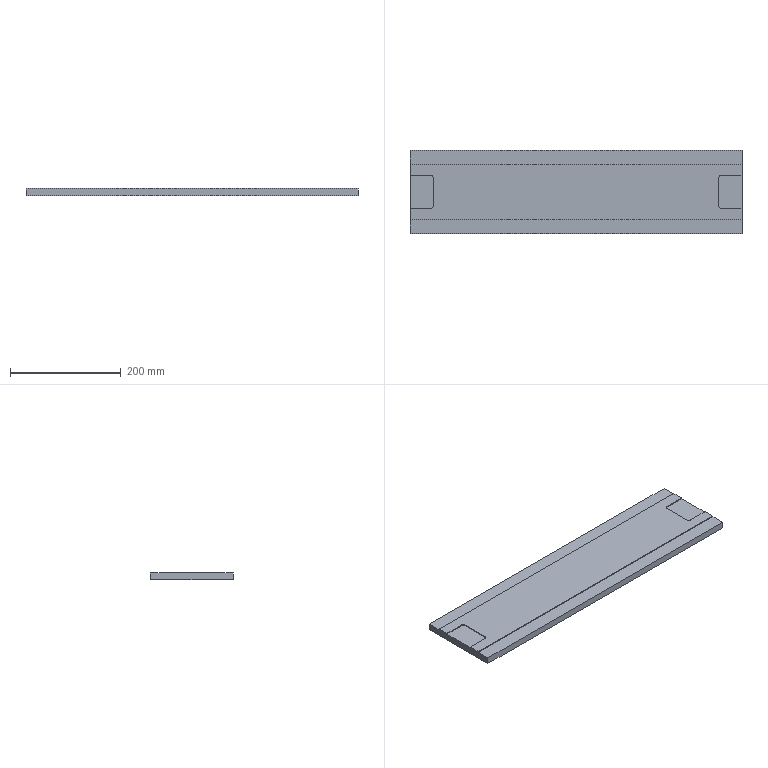Part | SolidWorks | features ICE 3, Extrusion 1, Fillet 1 | 1 solid | 22 faces | box 600 x 150 x 14 mm | volume 1207472 mm3 | plane 18 | cylinder 4 | commonest cylinder face diameters 10 x4
STEP:
#1=CARTESIAN_POINT('',(300.,75.,12.5));
#2=VERTEX_POINT('',#1);
#3=CARTESIAN_POINT('',(-300.,75.,12.5));
#4=VERTEX_POINT('',#3);
#5=CARTESIAN_POINT('',(-300.,75.,12.5));
#6=DIRECTION('',(-1.,0.,0.));
#7=VECTOR('',#6,1000.);
#8=LINE('',#5,#7);
#9=EDGE_CURVE('',#2,#4,#8,.T.);
#10=ORIENTED_EDGE('',*,*,#9,.F.);
#11=CARTESIAN_POINT('',(300.,75.,0.));
#12=VERTEX_POINT('',#11);
#13=CARTESIAN_POINT('',(300.,75.,14.));
#14=DIRECTION('',(0.,0.,-1.));
#15=VECTOR('',#14,1000.);
#16=LINE('',#13,#15);
#17=EDGE_CURVE('',#2,#12,#16,.T.);
#18=ORIENTED_EDGE('',*,*,#17,.T.);
#19=CARTESIAN_POINT('',(-300.,75.,0.));
#20=VERTEX_POINT('',#19);
#21=CARTESIAN_POINT('',(-300.,75.,0.));
#22=DIRECTION('',(-1.,0.,0.));
#23=VECTOR('',#22,1000.);
#24=LINE('',#21,#23);
#25=EDGE_CURVE('',#12,#20,#24,.T.);
#26=ORIENTED_EDGE('',*,*,#25,.T.);
#27=CARTESIAN_POINT('',(-300.,75.,14.));
#28=DIRECTION('',(0.,0.,-1.));
#29=VECTOR('',#28,1000.);
#30=LINE('',#27,#29);
#31=EDGE_CURVE('',#4,#20,#30,.T.);
#32=ORIENTED_EDGE('',*,*,#31,.F.);
#33=EDGE_LOOP('',(#10,#18,#26,#32));
#34=FACE_OUTER_BOUND('',#33,.T.);
#35=CARTESIAN_POINT('',(-300.,75.,14.));
#36=DIRECTION('',(0.,-1.,0.));
#37=DIRECTION('',(0.,0.,-1.));
#38=AXIS2_PLACEMENT_3D('',#35,#36,#37);
#39=PLANE('',#38);
#40=ADVANCED_FACE('',(#34),#39,.F.);
#41=CARTESIAN_POINT('',(300.,-30.,12.5));
#42=VERTEX_POINT('',#41);
#43=CARTESIAN_POINT('',(300.,30.,12.5));
#44=VERTEX_POINT('',#43);
#45=CARTESIAN_POINT('',(300.,-30.,12.5));
#46=DIRECTION('',(0.,1.,0.));
#47=VECTOR('',#46,1000.);
#48=LINE('',#45,#47);
#49=EDGE_CURVE('',#42,#44,#48,.T.);
#50=ORIENTED_EDGE('',*,*,#49,.F.);
#51=CARTESIAN_POINT('',(300.,-30.,14.));
#52=VERTEX_POINT('',#51);
#53=CARTESIAN_POINT('',(300.,-30.,12.5));
#54=DIRECTION('',(0.,0.,1.));
#55=VECTOR('',#54,1000.);
#56=LINE('',#53,#55);
#57=EDGE_CURVE('',#42,#52,#56,.T.);
#58=ORIENTED_EDGE('',*,*,#57,.T.);
#59=CARTESIAN_POINT('',(300.,-50.,14.));
#60=VERTEX_POINT('',#59);
#61=CARTESIAN_POINT('',(300.,-75.,14.));
#62=DIRECTION('',(0.,1.,0.));
#63=VECTOR('',#62,1000.);
#64=LINE('',#61,#63);
#65=EDGE_CURVE('',#60,#52,#64,.T.);
#66=ORIENTED_EDGE('',*,*,#65,.F.);
#67=CARTESIAN_POINT('',(300.,-50.,12.5));
#68=VERTEX_POINT('',#67);
#69=CARTESIAN_POINT('',(300.,-50.,12.5));
#70=DIRECTION('',(0.,0.,1.));
#71=VECTOR('',#70,1000.);
#72=LINE('',#69,#71);
#73=EDGE_CURVE('',#68,#60,#72,.T.);
#74=ORIENTED_EDGE('',*,*,#73,.F.);
#75=CARTESIAN_POINT('',(300.,-75.,12.5));
#76=VERTEX_POINT('',#75);
#77=CARTESIAN_POINT('',(300.,-75.,12.5));
#78=DIRECTION('',(0.,1.,0.));
#79=VECTOR('',#78,1000.);
#80=LINE('',#77,#79);
#81=EDGE_CURVE('',#76,#68,#80,.T.);
#82=ORIENTED_EDGE('',*,*,#81,.F.);
#83=CARTESIAN_POINT('',(300.,-75.,0.));
#84=VERTEX_POINT('',#83);
#85=CARTESIAN_POINT('',(300.,-75.,14.));
#86=DIRECTION('',(0.,0.,-1.));
#87=VECTOR('',#86,1000.);
#88=LINE('',#85,#87);
#89=EDGE_CURVE('',#76,#84,#88,.T.);
#90=ORIENTED_EDGE('',*,*,#89,.T.);
#91=CARTESIAN_POINT('',(300.,-75.,0.));
#92=DIRECTION('',(0.,1.,0.));
#93=VECTOR('',#92,1000.);
#94=LINE('',#91,#93);
#95=EDGE_CURVE('',#84,#12,#94,.T.);
#96=ORIENTED_EDGE('',*,*,#95,.T.);
#97=ORIENTED_EDGE('',*,*,#17,.F.);
#98=CARTESIAN_POINT('',(300.,50.,12.5));
#99=VERTEX_POINT('',#98);
#100=CARTESIAN_POINT('',(300.,75.,12.5));
#101=DIRECTION('',(0.,1.,0.));
#102=VECTOR('',#101,1000.);
#103=LINE('',#100,#102);
#104=EDGE_CURVE('',#99,#2,#103,.T.);
#105=ORIENTED_EDGE('',*,*,#104,.F.);
#106=CARTESIAN_POINT('',(300.,50.,14.));
#107=VERTEX_POINT('',#106);
#108=CARTESIAN_POINT('',(300.,50.,12.5));
#109=DIRECTION('',(0.,0.,1.));
#110=VECTOR('',#109,1000.);
#111=LINE('',#108,#110);
#112=EDGE_CURVE('',#99,#107,#111,.T.);
#113=ORIENTED_EDGE('',*,*,#112,.T.);
#114=CARTESIAN_POINT('',(300.,30.,14.));
#115=VERTEX_POINT('',#114);
#116=CARTESIAN_POINT('',(300.,-75.,14.));
#117=DIRECTION('',(0.,1.,0.));
#118=VECTOR('',#117,1000.);
#119=LINE('',#116,#118);
#120=EDGE_CURVE('',#115,#107,#119,.T.);
#121=ORIENTED_EDGE('',*,*,#120,.F.);
#122=CARTESIAN_POINT('',(300.,30.,12.5));
#123=DIRECTION('',(0.,0.,1.));
#124=VECTOR('',#123,1000.);
#125=LINE('',#122,#124);
#126=EDGE_CURVE('',#44,#115,#125,.T.);
#127=ORIENTED_EDGE('',*,*,#126,.F.);
#128=EDGE_LOOP('',(#50,#58,#66,#74,#82,#90,#96,#97,#105,#113,#121,#127));
#129=FACE_OUTER_BOUND('',#128,.T.);
#130=CARTESIAN_POINT('',(300.,-75.,14.));
#131=DIRECTION('',(-1.,0.,0.));
#132=DIRECTION('',(0.,0.,1.));
#133=AXIS2_PLACEMENT_3D('',#130,#131,#132);
#134=PLANE('',#133);
#135=ADVANCED_FACE('',(#129),#134,.F.);
#136=CARTESIAN_POINT('',(-300.,-30.,14.));
#137=VERTEX_POINT('',#136);
#138=CARTESIAN_POINT('',(-300.,-50.,14.));
#139=VERTEX_POINT('',#138);
#140=CARTESIAN_POINT('',(-300.,-75.,14.));
#141=DIRECTION('',(0.,-1.,0.));
#142=VECTOR('',#141,1000.);
#143=LINE('',#140,#142);
#144=EDGE_CURVE('',#137,#139,#143,.T.);
#145=ORIENTED_EDGE('',*,*,#144,.F.);
#146=CARTESIAN_POINT('',(-300.,-30.,12.5));
#147=VERTEX_POINT('',#146);
#148=CARTESIAN_POINT('',(-300.,-30.,12.5));
#149=DIRECTION('',(0.,0.,1.));
#150=VECTOR('',#149,1000.);
#151=LINE('',#148,#150);
#152=EDGE_CURVE('',#147,#137,#151,.T.);
#153=ORIENTED_EDGE('',*,*,#152,.F.);
#154=CARTESIAN_POINT('',(-300.,30.,12.5));
#155=VERTEX_POINT('',#154);
#156=CARTESIAN_POINT('',(-300.,-30.,12.5));
#157=DIRECTION('',(0.,-1.,0.));
#158=VECTOR('',#157,1000.);
#159=LINE('',#156,#158);
#160=EDGE_CURVE('',#155,#147,#159,.T.);
#161=ORIENTED_EDGE('',*,*,#160,.F.);
#162=CARTESIAN_POINT('',(-300.,30.,14.));
#163=VERTEX_POINT('',#162);
#164=CARTESIAN_POINT('',(-300.,30.,12.5));
#165=DIRECTION('',(0.,0.,1.));
#166=VECTOR('',#165,1000.);
#167=LINE('',#164,#166);
#168=EDGE_CURVE('',#155,#163,#167,.T.);
#169=ORIENTED_EDGE('',*,*,#168,.T.);
#170=CARTESIAN_POINT('',(-300.,50.,14.));
#171=VERTEX_POINT('',#170);
#172=CARTESIAN_POINT('',(-300.,-75.,14.));
#173=DIRECTION('',(0.,-1.,0.));
#174=VECTOR('',#173,1000.);
#175=LINE('',#172,#174);
#176=EDGE_CURVE('',#171,#163,#175,.T.);
#177=ORIENTED_EDGE('',*,*,#176,.F.);
#178=CARTESIAN_POINT('',(-300.,50.,12.5));
#179=VERTEX_POINT('',#178);
#180=CARTESIAN_POINT('',(-300.,50.,12.5));
#181=DIRECTION('',(0.,0.,1.));
#182=VECTOR('',#181,1000.);
#183=LINE('',#180,#182);
#184=EDGE_CURVE('',#179,#171,#183,.T.);
#185=ORIENTED_EDGE('',*,*,#184,.F.);
#186=CARTESIAN_POINT('',(-300.,75.,12.5));
#187=DIRECTION('',(0.,-1.,0.));
#188=VECTOR('',#187,1000.);
#189=LINE('',#186,#188);
#190=EDGE_CURVE('',#4,#179,#189,.T.);
#191=ORIENTED_EDGE('',*,*,#190,.F.);
#192=ORIENTED_EDGE('',*,*,#31,.T.);
#193=CARTESIAN_POINT('',(-300.,-75.,0.));
#194=VERTEX_POINT('',#193);
#195=CARTESIAN_POINT('',(-300.,-75.,0.));
#196=DIRECTION('',(0.,-1.,0.));
#197=VECTOR('',#196,1000.);
#198=LINE('',#195,#197);
#199=EDGE_CURVE('',#20,#194,#198,.T.);
#200=ORIENTED_EDGE('',*,*,#199,.T.);
#201=CARTESIAN_POINT('',(-300.,-75.,12.5));
#202=VERTEX_POINT('',#201);
#203=CARTESIAN_POINT('',(-300.,-75.,14.));
#204=DIRECTION('',(0.,0.,-1.));
#205=VECTOR('',#204,1000.);
#206=LINE('',#203,#205);
#207=EDGE_CURVE('',#202,#194,#206,.T.);
#208=ORIENTED_EDGE('',*,*,#207,.F.);
#209=CARTESIAN_POINT('',(-300.,-50.,12.5));
#210=VERTEX_POINT('',#209);
#211=CARTESIAN_POINT('',(-300.,-75.,12.5));
#212=DIRECTION('',(0.,-1.,0.));
#213=VECTOR('',#212,1000.);
#214=LINE('',#211,#213);
#215=EDGE_CURVE('',#210,#202,#214,.T.);
#216=ORIENTED_EDGE('',*,*,#215,.F.);
#217=CARTESIAN_POINT('',(-300.,-50.,12.5));
#218=DIRECTION('',(0.,0.,1.));
#219=VECTOR('',#218,1000.);
#220=LINE('',#217,#219);
#221=EDGE_CURVE('',#210,#139,#220,.T.);
#222=ORIENTED_EDGE('',*,*,#221,.T.);
#223=EDGE_LOOP('',(#145,#153,#161,#169,#177,#185,#191,#192,#200,#208,#216,#222));
#224=FACE_OUTER_BOUND('',#223,.T.);
#225=CARTESIAN_POINT('',(-300.,-75.,14.));
#226=DIRECTION('',(1.,0.,0.));
#227=DIRECTION('',(0.,0.,-1.));
#228=AXIS2_PLACEMENT_3D('',#225,#226,#227);
#229=PLANE('',#228);
#230=ADVANCED_FACE('',(#224),#229,.F.);
#231=ORIENTED_EDGE('',*,*,#89,.F.);
#232=CARTESIAN_POINT('',(-300.,-75.,12.5));
#233=DIRECTION('',(1.,0.,0.));
#234=VECTOR('',#233,1000.);
#235=LINE('',#232,#234);
#236=EDGE_CURVE('',#202,#76,#235,.T.);
#237=ORIENTED_EDGE('',*,*,#236,.F.);
#238=ORIENTED_EDGE('',*,*,#207,.T.);
#239=CARTESIAN_POINT('',(-300.,-75.,0.));
#240=DIRECTION('',(1.,0.,0.));
#241=VECTOR('',#240,1000.);
#242=LINE('',#239,#241);
#243=EDGE_CURVE('',#194,#84,#242,.T.);
#244=ORIENTED_EDGE('',*,*,#243,.T.);
#245=EDGE_LOOP('',(#231,#237,#238,#244));
#246=FACE_OUTER_BOUND('',#245,.T.);
#247=CARTESIAN_POINT('',(-300.,-75.,14.));
#248=DIRECTION('',(0.,1.,0.));
#249=DIRECTION('',(0.,0.,1.));
#250=AXIS2_PLACEMENT_3D('',#247,#248,#249);
#251=PLANE('',#250);
#252=ADVANCED_FACE('',(#246),#251,.F.);
#253=CARTESIAN_POINT('',(-258.,-25.,14.));
#254=VERTEX_POINT('',#253);
#255=CARTESIAN_POINT('',(-258.,25.,14.));
#256=VERTEX_POINT('',#255);
#257=CARTESIAN_POINT('',(-258.,-30.,14.));
#258=DIRECTION('',(0.,1.,0.));
#259=VECTOR('',#258,1000.);
#260=LINE('',#257,#259);
#261=EDGE_CURVE('',#254,#256,#260,.T.);
#262=ORIENTED_EDGE('',*,*,#261,.F.);
#263=CARTESIAN_POINT('',(-263.,-30.,14.));
#264=VERTEX_POINT('',#263);
#265=CARTESIAN_POINT('',(-263.,-25.,14.));
#266=DIRECTION('',(0.,0.,-1.));
#267=DIRECTION('',(-1.,0.,0.));
#268=AXIS2_PLACEMENT_3D('',#265,#266,#267);
#269=CIRCLE('',#268,5.);
#270=EDGE_CURVE('',#254,#264,#269,.T.);
#271=ORIENTED_EDGE('',*,*,#270,.T.);
#272=CARTESIAN_POINT('',(-300.,-30.,14.));
#273=DIRECTION('',(1.,0.,0.));
#274=VECTOR('',#273,1000.);
#275=LINE('',#272,#274);
#276=EDGE_CURVE('',#137,#264,#275,.T.);
#277=ORIENTED_EDGE('',*,*,#276,.F.);
#278=ORIENTED_EDGE('',*,*,#144,.T.);
#279=CARTESIAN_POINT('',(-300.,-50.,14.));
#280=DIRECTION('',(-1.,0.,0.));
#281=VECTOR('',#280,1000.);
#282=LINE('',#279,#281);
#283=EDGE_CURVE('',#60,#139,#282,.T.);
#284=ORIENTED_EDGE('',*,*,#283,.F.);
#285=ORIENTED_EDGE('',*,*,#65,.T.);
#286=CARTESIAN_POINT('',(263.,-30.,14.));
#287=VERTEX_POINT('',#286);
#288=CARTESIAN_POINT('',(258.,-30.,14.));
#289=DIRECTION('',(1.,0.,0.));
#290=VECTOR('',#289,1000.);
#291=LINE('',#288,#290);
#292=EDGE_CURVE('',#287,#52,#291,.T.);
#293=ORIENTED_EDGE('',*,*,#292,.F.);
#294=CARTESIAN_POINT('',(258.,-25.,14.));
#295=VERTEX_POINT('',#294);
#296=CARTESIAN_POINT('',(263.,-25.,14.));
#297=DIRECTION('',(0.,0.,-1.));
#298=DIRECTION('',(-1.,0.,0.));
#299=AXIS2_PLACEMENT_3D('',#296,#297,#298);
#300=CIRCLE('',#299,5.);
#301=EDGE_CURVE('',#287,#295,#300,.T.);
#302=ORIENTED_EDGE('',*,*,#301,.T.);
#303=CARTESIAN_POINT('',(258.,25.,14.));
#304=VERTEX_POINT('',#303);
#305=CARTESIAN_POINT('',(258.,-30.,14.));
#306=DIRECTION('',(0.,-1.,0.));
#307=VECTOR('',#306,1000.);
#308=LINE('',#305,#307);
#309=EDGE_CURVE('',#304,#295,#308,.T.);
#310=ORIENTED_EDGE('',*,*,#309,.F.);
#311=CARTESIAN_POINT('',(263.,30.,14.));
#312=VERTEX_POINT('',#311);
#313=CARTESIAN_POINT('',(263.,25.,14.));
#314=DIRECTION('',(0.,0.,-1.));
#315=DIRECTION('',(-1.,0.,0.));
#316=AXIS2_PLACEMENT_3D('',#313,#314,#315);
#317=CIRCLE('',#316,5.);
#318=EDGE_CURVE('',#304,#312,#317,.T.);
#319=ORIENTED_EDGE('',*,*,#318,.T.);
#320=CARTESIAN_POINT('',(258.,30.,14.));
#321=DIRECTION('',(-1.,0.,0.));
#322=VECTOR('',#321,1000.);
#323=LINE('',#320,#322);
#324=EDGE_CURVE('',#115,#312,#323,.T.);
#325=ORIENTED_EDGE('',*,*,#324,.F.);
#326=ORIENTED_EDGE('',*,*,#120,.T.);
#327=CARTESIAN_POINT('',(-300.,50.,14.));
#328=DIRECTION('',(1.,0.,0.));
#329=VECTOR('',#328,1000.);
#330=LINE('',#327,#329);
#331=EDGE_CURVE('',#171,#107,#330,.T.);
#332=ORIENTED_EDGE('',*,*,#331,.F.);
#333=ORIENTED_EDGE('',*,*,#176,.T.);
#334=CARTESIAN_POINT('',(-263.,30.,14.));
#335=VERTEX_POINT('',#334);
#336=CARTESIAN_POINT('',(-300.,30.,14.));
#337=DIRECTION('',(-1.,0.,0.));
#338=VECTOR('',#337,1000.);
#339=LINE('',#336,#338);
#340=EDGE_CURVE('',#335,#163,#339,.T.);
#341=ORIENTED_EDGE('',*,*,#340,.F.);
#342=CARTESIAN_POINT('',(-263.,25.,14.));
#343=DIRECTION('',(0.,0.,-1.));
#344=DIRECTION('',(-1.,0.,0.));
#345=AXIS2_PLACEMENT_3D('',#342,#343,#344);
#346=CIRCLE('',#345,5.);
#347=EDGE_CURVE('',#335,#256,#346,.T.);
#348=ORIENTED_EDGE('',*,*,#347,.T.);
#349=EDGE_LOOP('',(#262,#271,#277,#278,#284,#285,#293,#302,#310,#319,#325,#326,#332,#333,#341,#348));
#350=FACE_OUTER_BOUND('',#349,.T.);
#351=CARTESIAN_POINT('',(0.,0.,14.));
#352=DIRECTION('',(0.,0.,-1.));
#353=DIRECTION('',(-1.,0.,0.));
#354=AXIS2_PLACEMENT_3D('',#351,#352,#353);
#355=PLANE('',#354);
#356=ADVANCED_FACE('',(#350),#355,.F.);
#357=ORIENTED_EDGE('',*,*,#95,.F.);
#358=ORIENTED_EDGE('',*,*,#243,.F.);
#359=ORIENTED_EDGE('',*,*,#199,.F.);
#360=ORIENTED_EDGE('',*,*,#25,.F.);
#361=EDGE_LOOP('',(#357,#358,#359,#360));
#362=FACE_OUTER_BOUND('',#361,.T.);
#363=CARTESIAN_POINT('',(0.,0.,0.));
#364=DIRECTION('',(0.,0.,-1.));
#365=DIRECTION('',(-1.,0.,0.));
#366=AXIS2_PLACEMENT_3D('',#363,#364,#365);
#367=PLANE('',#366);
#368=ADVANCED_FACE('',(#362),#367,.T.);
#369=ORIENTED_EDGE('',*,*,#283,.T.);
#370=ORIENTED_EDGE('',*,*,#221,.F.);
#371=CARTESIAN_POINT('',(-300.,-50.,12.5));
#372=DIRECTION('',(-1.,0.,0.));
#373=VECTOR('',#372,1000.);
#374=LINE('',#371,#373);
#375=EDGE_CURVE('',#68,#210,#374,.T.);
#376=ORIENTED_EDGE('',*,*,#375,.F.);
#377=ORIENTED_EDGE('',*,*,#73,.T.);
#378=EDGE_LOOP('',(#369,#370,#376,#377));
#379=FACE_OUTER_BOUND('',#378,.T.);
#380=CARTESIAN_POINT('',(-300.,-50.,12.5));
#381=DIRECTION('',(0.,1.,0.));
#382=DIRECTION('',(-1.,0.,0.));
#383=AXIS2_PLACEMENT_3D('',#380,#381,#382);
#384=PLANE('',#383);
#385=ADVANCED_FACE('',(#379),#384,.F.);
#386=ORIENTED_EDGE('',*,*,#215,.T.);
#387=ORIENTED_EDGE('',*,*,#236,.T.);
#388=ORIENTED_EDGE('',*,*,#81,.T.);
#389=ORIENTED_EDGE('',*,*,#375,.T.);
#390=EDGE_LOOP('',(#386,#387,#388,#389));
#391=FACE_OUTER_BOUND('',#390,.T.);
#392=CARTESIAN_POINT('',(0.,0.,12.5));
#393=DIRECTION('',(0.,0.,-1.));
#394=DIRECTION('',(-1.,0.,0.));
#395=AXIS2_PLACEMENT_3D('',#392,#393,#394);
#396=PLANE('',#395);
#397=ADVANCED_FACE('',(#391),#396,.F.);
#398=ORIENTED_EDGE('',*,*,#331,.T.);
#399=ORIENTED_EDGE('',*,*,#112,.F.);
#400=CARTESIAN_POINT('',(-300.,50.,12.5));
#401=DIRECTION('',(1.,0.,0.));
#402=VECTOR('',#401,1000.);
#403=LINE('',#400,#402);
#404=EDGE_CURVE('',#179,#99,#403,.T.);
#405=ORIENTED_EDGE('',*,*,#404,.F.);
#406=ORIENTED_EDGE('',*,*,#184,.T.);
#407=EDGE_LOOP('',(#398,#399,#405,#406));
#408=FACE_OUTER_BOUND('',#407,.T.);
#409=CARTESIAN_POINT('',(-300.,50.,12.5));
#410=DIRECTION('',(0.,-1.,0.));
#411=DIRECTION('',(0.,0.,-1.));
#412=AXIS2_PLACEMENT_3D('',#409,#410,#411);
#413=PLANE('',#412);
#414=ADVANCED_FACE('',(#408),#413,.F.);
#415=ORIENTED_EDGE('',*,*,#190,.T.);
#416=ORIENTED_EDGE('',*,*,#404,.T.);
#417=ORIENTED_EDGE('',*,*,#104,.T.);
#418=ORIENTED_EDGE('',*,*,#9,.T.);
#419=EDGE_LOOP('',(#415,#416,#417,#418));
#420=FACE_OUTER_BOUND('',#419,.T.);
#421=CARTESIAN_POINT('',(0.,0.,12.5));
#422=DIRECTION('',(0.,0.,1.));
#423=DIRECTION('',(1.,0.,0.));
#424=AXIS2_PLACEMENT_3D('',#421,#422,#423);
#425=PLANE('',#424);
#426=ADVANCED_FACE('',(#420),#425,.T.);
#427=CARTESIAN_POINT('',(263.,-30.,12.5));
#428=VERTEX_POINT('',#427);
#429=CARTESIAN_POINT('',(258.,-30.,12.5));
#430=DIRECTION('',(1.,0.,0.));
#431=VECTOR('',#430,1000.);
#432=LINE('',#429,#431);
#433=EDGE_CURVE('',#428,#42,#432,.T.);
#434=ORIENTED_EDGE('',*,*,#433,.F.);
#435=CARTESIAN_POINT('',(263.,-30.,14.));
#436=DIRECTION('',(0.,0.,1.));
#437=VECTOR('',#436,1000.);
#438=LINE('',#435,#437);
#439=EDGE_CURVE('',#428,#287,#438,.T.);
#440=ORIENTED_EDGE('',*,*,#439,.T.);
#441=ORIENTED_EDGE('',*,*,#292,.T.);
#442=ORIENTED_EDGE('',*,*,#57,.F.);
#443=EDGE_LOOP('',(#434,#440,#441,#442));
#444=FACE_OUTER_BOUND('',#443,.T.);
#445=CARTESIAN_POINT('',(258.,-30.,12.5));
#446=DIRECTION('',(0.,-1.,0.));
#447=DIRECTION('',(1.,0.,0.));
#448=AXIS2_PLACEMENT_3D('',#445,#446,#447);
#449=PLANE('',#448);
#450=ADVANCED_FACE('',(#444),#449,.F.);
#451=ORIENTED_EDGE('',*,*,#309,.T.);
#452=CARTESIAN_POINT('',(258.,-25.,12.5));
#453=VERTEX_POINT('',#452);
#454=CARTESIAN_POINT('',(258.,-25.,12.5));
#455=DIRECTION('',(0.,0.,-1.));
#456=VECTOR('',#455,1000.);
#457=LINE('',#454,#456);
#458=EDGE_CURVE('',#295,#453,#457,.T.);
#459=ORIENTED_EDGE('',*,*,#458,.T.);
#460=CARTESIAN_POINT('',(258.,25.,12.5));
#461=VERTEX_POINT('',#460);
#462=CARTESIAN_POINT('',(258.,-30.,12.5));
#463=DIRECTION('',(0.,-1.,0.));
#464=VECTOR('',#463,1000.);
#465=LINE('',#462,#464);
#466=EDGE_CURVE('',#461,#453,#465,.T.);
#467=ORIENTED_EDGE('',*,*,#466,.F.);
#468=CARTESIAN_POINT('',(258.,25.,14.));
#469=DIRECTION('',(0.,0.,1.));
#470=VECTOR('',#469,1000.);
#471=LINE('',#468,#470);
#472=EDGE_CURVE('',#461,#304,#471,.T.);
#473=ORIENTED_EDGE('',*,*,#472,.T.);
#474=EDGE_LOOP('',(#451,#459,#467,#473));
#475=FACE_OUTER_BOUND('',#474,.T.);
#476=CARTESIAN_POINT('',(258.,-30.,12.5));
#477=DIRECTION('',(-1.,0.,0.));
#478=DIRECTION('',(0.,0.,1.));
#479=AXIS2_PLACEMENT_3D('',#476,#477,#478);
#480=PLANE('',#479);
#481=ADVANCED_FACE('',(#475),#480,.F.);
#482=ORIENTED_EDGE('',*,*,#324,.T.);
#483=CARTESIAN_POINT('',(263.,30.,12.5));
#484=VERTEX_POINT('',#483);
#485=CARTESIAN_POINT('',(263.,30.,12.5));
#486=DIRECTION('',(0.,0.,-1.));
#487=VECTOR('',#486,1000.);
#488=LINE('',#485,#487);
#489=EDGE_CURVE('',#312,#484,#488,.T.);
#490=ORIENTED_EDGE('',*,*,#489,.T.);
#491=CARTESIAN_POINT('',(258.,30.,12.5));
#492=DIRECTION('',(-1.,0.,0.));
#493=VECTOR('',#492,1000.);
#494=LINE('',#491,#493);
#495=EDGE_CURVE('',#44,#484,#494,.T.);
#496=ORIENTED_EDGE('',*,*,#495,.F.);
#497=ORIENTED_EDGE('',*,*,#126,.T.);
#498=EDGE_LOOP('',(#482,#490,#496,#497));
#499=FACE_OUTER_BOUND('',#498,.T.);
#500=CARTESIAN_POINT('',(258.,30.,12.5));
#501=DIRECTION('',(0.,1.,0.));
#502=DIRECTION('',(0.,0.,1.));
#503=AXIS2_PLACEMENT_3D('',#500,#501,#502);
#504=PLANE('',#503);
#505=ADVANCED_FACE('',(#499),#504,.F.);
#506=ORIENTED_EDGE('',*,*,#466,.T.);
#507=CARTESIAN_POINT('',(263.,-25.,12.5));
#508=DIRECTION('',(0.,0.,1.));
#509=DIRECTION('',(-1.,0.,0.));
#510=AXIS2_PLACEMENT_3D('',#507,#508,#509);
#511=CIRCLE('',#510,5.);
#512=EDGE_CURVE('',#453,#428,#511,.T.);
#513=ORIENTED_EDGE('',*,*,#512,.T.);
#514=ORIENTED_EDGE('',*,*,#433,.T.);
#515=ORIENTED_EDGE('',*,*,#49,.T.);
#516=ORIENTED_EDGE('',*,*,#495,.T.);
#517=CARTESIAN_POINT('',(263.,25.,12.5));
#518=DIRECTION('',(0.,0.,1.));
#519=DIRECTION('',(-1.,0.,0.));
#520=AXIS2_PLACEMENT_3D('',#517,#518,#519);
#521=CIRCLE('',#520,5.);
#522=EDGE_CURVE('',#484,#461,#521,.T.);
#523=ORIENTED_EDGE('',*,*,#522,.T.);
#524=EDGE_LOOP('',(#506,#513,#514,#515,#516,#523));
#525=FACE_OUTER_BOUND('',#524,.T.);
#526=CARTESIAN_POINT('',(0.,0.,12.5));
#527=DIRECTION('',(0.,0.,-1.));
#528=DIRECTION('',(-1.,0.,0.));
#529=AXIS2_PLACEMENT_3D('',#526,#527,#528);
#530=PLANE('',#529);
#531=ADVANCED_FACE('',(#525),#530,.F.);
#532=CARTESIAN_POINT('',(-258.,-25.,12.5));
#533=VERTEX_POINT('',#532);
#534=CARTESIAN_POINT('',(-258.,25.,12.5));
#535=VERTEX_POINT('',#534);
#536=CARTESIAN_POINT('',(-258.,-30.,12.5));
#537=DIRECTION('',(0.,1.,0.));
#538=VECTOR('',#537,1000.);
#539=LINE('',#536,#538);
#540=EDGE_CURVE('',#533,#535,#539,.T.);
#541=ORIENTED_EDGE('',*,*,#540,.F.);
#542=CARTESIAN_POINT('',(-258.,-25.,14.));
#543=DIRECTION('',(0.,0.,1.));
#544=VECTOR('',#543,1000.);
#545=LINE('',#542,#544);
#546=EDGE_CURVE('',#533,#254,#545,.T.);
#547=ORIENTED_EDGE('',*,*,#546,.T.);
#548=ORIENTED_EDGE('',*,*,#261,.T.);
#549=CARTESIAN_POINT('',(-258.,25.,12.5));
#550=DIRECTION('',(0.,0.,-1.));
#551=VECTOR('',#550,1000.);
#552=LINE('',#549,#551);
#553=EDGE_CURVE('',#256,#535,#552,.T.);
#554=ORIENTED_EDGE('',*,*,#553,.T.);
#555=EDGE_LOOP('',(#541,#547,#548,#554));
#556=FACE_OUTER_BOUND('',#555,.T.);
#557=CARTESIAN_POINT('',(-258.,-30.,12.5));
#558=DIRECTION('',(1.,0.,0.));
#559=DIRECTION('',(0.,0.,-1.));
#560=AXIS2_PLACEMENT_3D('',#557,#558,#559);
#561=PLANE('',#560);
#562=ADVANCED_FACE('',(#556),#561,.F.);
#563=ORIENTED_EDGE('',*,*,#276,.T.);
#564=CARTESIAN_POINT('',(-263.,-30.,12.5));
#565=VERTEX_POINT('',#564);
#566=CARTESIAN_POINT('',(-263.,-30.,12.5));
#567=DIRECTION('',(0.,0.,-1.));
#568=VECTOR('',#567,1000.);
#569=LINE('',#566,#568);
#570=EDGE_CURVE('',#264,#565,#569,.T.);
#571=ORIENTED_EDGE('',*,*,#570,.T.);
#572=CARTESIAN_POINT('',(-300.,-30.,12.5));
#573=DIRECTION('',(1.,0.,0.));
#574=VECTOR('',#573,1000.);
#575=LINE('',#572,#574);
#576=EDGE_CURVE('',#147,#565,#575,.T.);
#577=ORIENTED_EDGE('',*,*,#576,.F.);
#578=ORIENTED_EDGE('',*,*,#152,.T.);
#579=EDGE_LOOP('',(#563,#571,#577,#578));
#580=FACE_OUTER_BOUND('',#579,.T.);
#581=CARTESIAN_POINT('',(-300.,-30.,12.5));
#582=DIRECTION('',(0.,-1.,0.));
#583=DIRECTION('',(0.,0.,-1.));
#584=AXIS2_PLACEMENT_3D('',#581,#582,#583);
#585=PLANE('',#584);
#586=ADVANCED_FACE('',(#580),#585,.F.);
#587=CARTESIAN_POINT('',(-263.,30.,12.5));
#588=VERTEX_POINT('',#587);
#589=CARTESIAN_POINT('',(-300.,30.,12.5));
#590=DIRECTION('',(-1.,0.,0.));
#591=VECTOR('',#590,1000.);
#592=LINE('',#589,#591);
#593=EDGE_CURVE('',#588,#155,#592,.T.);
#594=ORIENTED_EDGE('',*,*,#593,.F.);
#595=CARTESIAN_POINT('',(-263.,30.,14.));
#596=DIRECTION('',(0.,0.,1.));
#597=VECTOR('',#596,1000.);
#598=LINE('',#595,#597);
#599=EDGE_CURVE('',#588,#335,#598,.T.);
#600=ORIENTED_EDGE('',*,*,#599,.T.);
#601=ORIENTED_EDGE('',*,*,#340,.T.);
#602=ORIENTED_EDGE('',*,*,#168,.F.);
#603=EDGE_LOOP('',(#594,#600,#601,#602));
#604=FACE_OUTER_BOUND('',#603,.T.);
#605=CARTESIAN_POINT('',(-300.,30.,12.5));
#606=DIRECTION('',(0.,1.,0.));
#607=DIRECTION('',(0.,0.,1.));
#608=AXIS2_PLACEMENT_3D('',#605,#606,#607);
#609=PLANE('',#608);
#610=ADVANCED_FACE('',(#604),#609,.F.);
#611=ORIENTED_EDGE('',*,*,#576,.T.);
#612=CARTESIAN_POINT('',(-263.,-25.,12.5));
#613=DIRECTION('',(0.,0.,1.));
#614=DIRECTION('',(-1.,0.,0.));
#615=AXIS2_PLACEMENT_3D('',#612,#613,#614);
#616=CIRCLE('',#615,5.);
#617=EDGE_CURVE('',#565,#533,#616,.T.);
#618=ORIENTED_EDGE('',*,*,#617,.T.);
#619=ORIENTED_EDGE('',*,*,#540,.T.);
#620=CARTESIAN_POINT('',(-263.,25.,12.5));
#621=DIRECTION('',(0.,0.,1.));
#622=DIRECTION('',(-1.,0.,0.));
#623=AXIS2_PLACEMENT_3D('',#620,#621,#622);
#624=CIRCLE('',#623,5.);
#625=EDGE_CURVE('',#535,#588,#624,.T.);
#626=ORIENTED_EDGE('',*,*,#625,.T.);
#627=ORIENTED_EDGE('',*,*,#593,.T.);
#628=ORIENTED_EDGE('',*,*,#160,.T.);
#629=EDGE_LOOP('',(#611,#618,#619,#626,#627,#628));
#630=FACE_OUTER_BOUND('',#629,.T.);
#631=CARTESIAN_POINT('',(0.,0.,12.5));
#632=DIRECTION('',(0.,0.,-1.));
#633=DIRECTION('',(-1.,0.,0.));
#634=AXIS2_PLACEMENT_3D('',#631,#632,#633);
#635=PLANE('',#634);
#636=ADVANCED_FACE('',(#630),#635,.F.);
#637=ORIENTED_EDGE('',*,*,#512,.F.);
#638=ORIENTED_EDGE('',*,*,#458,.F.);
#639=ORIENTED_EDGE('',*,*,#301,.F.);
#640=ORIENTED_EDGE('',*,*,#439,.F.);
#641=EDGE_LOOP('',(#637,#638,#639,#640));
#642=FACE_OUTER_BOUND('',#641,.T.);
#643=CARTESIAN_POINT('',(263.,-25.,12.5));
#644=DIRECTION('',(0.,0.,-1.));
#645=DIRECTION('',(-1.,0.,0.));
#646=AXIS2_PLACEMENT_3D('',#643,#644,#645);
#647=CYLINDRICAL_SURFACE('',#646,5.);
#648=ADVANCED_FACE('',(#642),#647,.F.);
#649=ORIENTED_EDGE('',*,*,#522,.F.);
#650=ORIENTED_EDGE('',*,*,#489,.F.);
#651=ORIENTED_EDGE('',*,*,#318,.F.);
#652=ORIENTED_EDGE('',*,*,#472,.F.);
#653=EDGE_LOOP('',(#649,#650,#651,#652));
#654=FACE_OUTER_BOUND('',#653,.T.);
#655=CARTESIAN_POINT('',(263.,25.,12.5));
#656=DIRECTION('',(0.,0.,-1.));
#657=DIRECTION('',(-1.,0.,0.));
#658=AXIS2_PLACEMENT_3D('',#655,#656,#657);
#659=CYLINDRICAL_SURFACE('',#658,5.);
#660=ADVANCED_FACE('',(#654),#659,.F.);
#661=ORIENTED_EDGE('',*,*,#617,.F.);
#662=ORIENTED_EDGE('',*,*,#570,.F.);
#663=ORIENTED_EDGE('',*,*,#270,.F.);
#664=ORIENTED_EDGE('',*,*,#546,.F.);
#665=EDGE_LOOP('',(#661,#662,#663,#664));
#666=FACE_OUTER_BOUND('',#665,.T.);
#667=CARTESIAN_POINT('',(-263.,-25.,12.5));
#668=DIRECTION('',(0.,0.,-1.));
#669=DIRECTION('',(-1.,0.,0.));
#670=AXIS2_PLACEMENT_3D('',#667,#668,#669);
#671=CYLINDRICAL_SURFACE('',#670,5.);
#672=ADVANCED_FACE('',(#666),#671,.F.);
#673=ORIENTED_EDGE('',*,*,#625,.F.);
#674=ORIENTED_EDGE('',*,*,#553,.F.);
#675=ORIENTED_EDGE('',*,*,#347,.F.);
#676=ORIENTED_EDGE('',*,*,#599,.F.);
#677=EDGE_LOOP('',(#673,#674,#675,#676));
#678=FACE_OUTER_BOUND('',#677,.T.);
#679=CARTESIAN_POINT('',(-263.,25.,12.5));
#680=DIRECTION('',(0.,0.,-1.));
#681=DIRECTION('',(-1.,0.,0.));
#682=AXIS2_PLACEMENT_3D('',#679,#680,#681);
#683=CYLINDRICAL_SURFACE('',#682,5.);
#684=ADVANCED_FACE('',(#678),#683,.F.);
#685=CLOSED_SHELL('',(#40,#135,#230,#252,#356,#368,#385,#397,#414,#426,#450,#481,#505,#531,#562,#586,#610,#636,#648,#660,#672,#684));
#686=MANIFOLD_SOLID_BREP('',#685);
#687=CARTESIAN_POINT('',(0.,0.,0.));
#688=DIRECTION('',(0.,0.,1.));
#689=DIRECTION('',(1.,0.,0.));
#690=AXIS2_PLACEMENT_3D('',#687,#688,#689);
#691=(LENGTH_UNIT()NAMED_UNIT(*)SI_UNIT(.MILLI.,.METRE.));
#692=UNCERTAINTY_MEASURE_WITH_UNIT(LENGTH_MEASURE(0.00001),#691,'','');
#693=(NAMED_UNIT(*)PLANE_ANGLE_UNIT()SI_UNIT($,.RADIAN.));
#694=(NAMED_UNIT(*)SI_UNIT($,.STERADIAN.)SOLID_ANGLE_UNIT());
#695=(GEOMETRIC_REPRESENTATION_CONTEXT(3)GLOBAL_UNCERTAINTY_ASSIGNED_CONTEXT((#692))GLOBAL_UNIT_ASSIGNED_CONTEXT((#691,#693,#694))REPRESENTATION_CONTEXT('',''));
#696=ADVANCED_BREP_SHAPE_REPRESENTATION('',(#686,#690),#695);